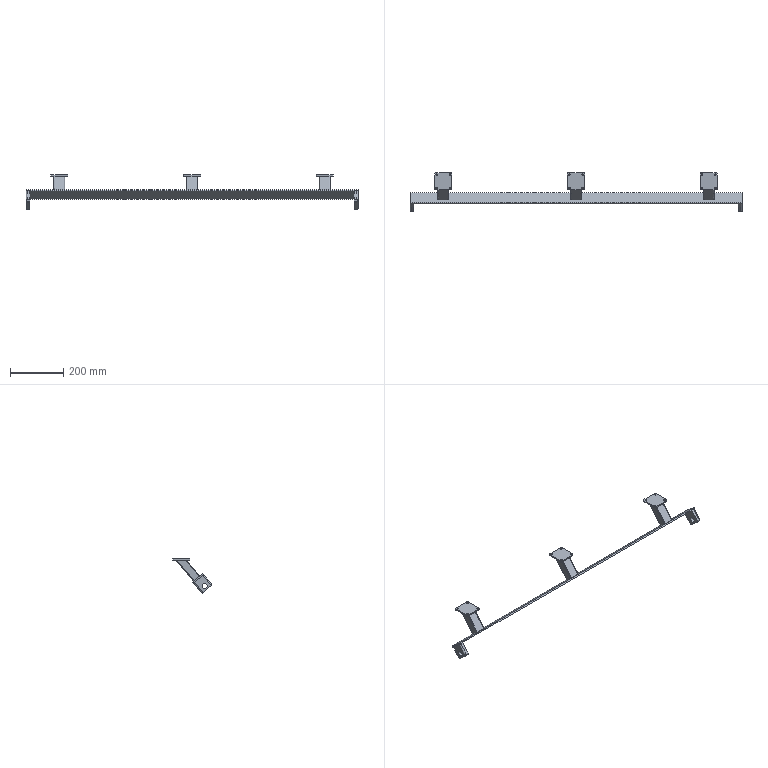Part | SolidWorks | features ICE 5, Fillet 2, Extrusion 1, LPattern 1, Sweep 1 | 6 solids | 138 faces | box 1250 x 145.623 x 130.346 mm | volume 500895 mm3 | plane 68 | cylinder 46 | spline 24 | commonest cylinder face diameters 5.2 x24 10 x18 20 x4